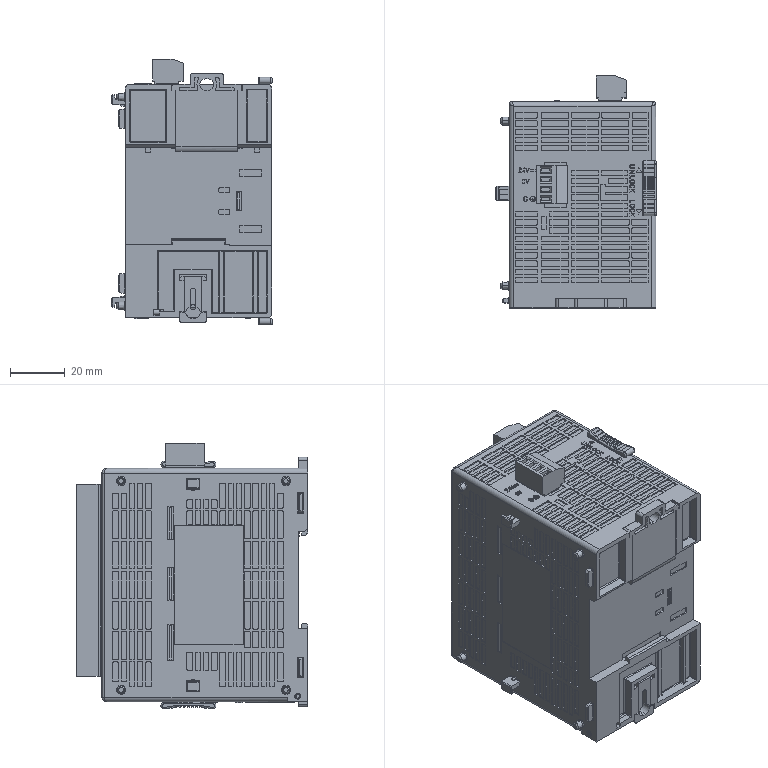Part | SolidWorks | features BaseBody 1 | 1 solid | 5943 faces | volume 331600 mm3 | plane 3998 | cylinder 1772 | cone 127 | torus 19 | sphere 18 | spline 9 | commonest cylinder face diameters 0.4 x1393 1 x87 0.6 x76 2.6 x72 2.8 x52 5.6 x24